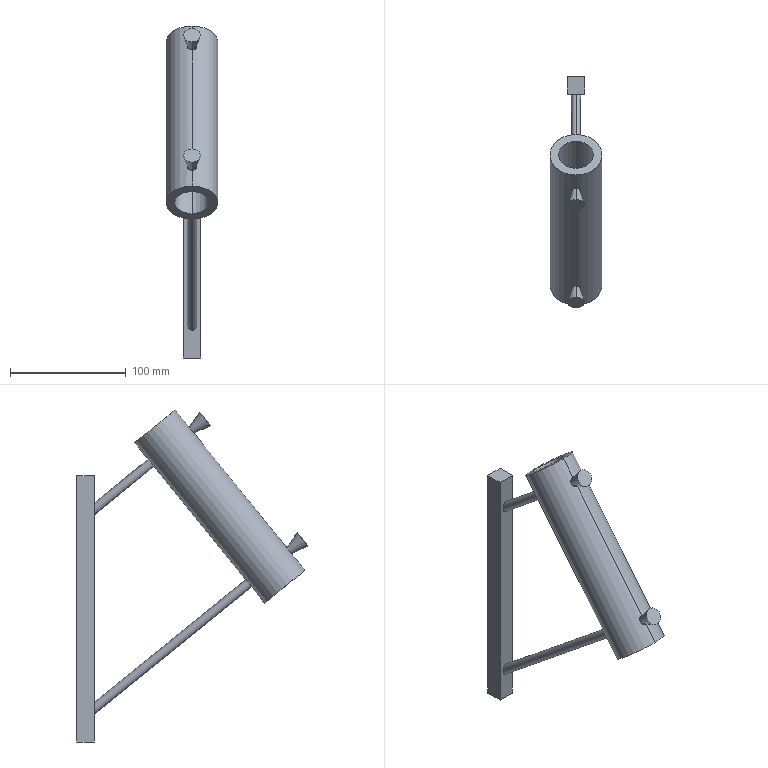Part | SolidWorks | features ICE 7, Cut 1, Extrusion 1 | 1 solid | 34 faces | box 45 x 200.096 x 286.61 mm | volume 222734 mm3 | cylinder 16 | plane 14 | cone 4 | commonest cylinder face diameters 8 x5 8.4 x4 8.2 x2 30 x2 45 x2 8.948 x1
STEP:
#1=CARTESIAN_POINT('',(-7.5,-176.098,143.559));
#2=VERTEX_POINT('',#1);
#3=CARTESIAN_POINT('',(-7.5,-152.784,124.679));
#4=VERTEX_POINT('',#3);
#5=CARTESIAN_POINT('',(-7.5,-164.441,134.119));
#6=DIRECTION('',(0.,-0.6293,-0.7771));
#7=DIRECTION('',(0.,0.7771,-0.6293));
#8=AXIS2_PLACEMENT_3D('',#5,#6,#7);
#9=CIRCLE('',#8,15.);
#10=EDGE_CURVE('',#2,#4,#9,.T.);
#11=ORIENTED_EDGE('',*,*,#10,.T.);
#12=CARTESIAN_POINT('',(-7.5,-40.765,263.011));
#13=VERTEX_POINT('',#12);
#14=CARTESIAN_POINT('',(-7.5,-162.224,113.022));
#15=DIRECTION('',(0.,0.6293,0.7771));
#16=VECTOR('',#15,1000.);
#17=LINE('',#14,#16);
#18=EDGE_CURVE('',#4,#13,#17,.T.);
#19=ORIENTED_EDGE('',*,*,#18,.T.);
#20=CARTESIAN_POINT('',(-7.5,-64.079,281.891));
#21=VERTEX_POINT('',#20);
#22=CARTESIAN_POINT('',(-7.5,-52.422,272.451));
#23=DIRECTION('',(0.,0.6293,0.7771));
#24=DIRECTION('',(0.,-0.7771,0.6293));
#25=AXIS2_PLACEMENT_3D('',#22,#23,#24);
#26=CIRCLE('',#25,15.);
#27=EDGE_CURVE('',#13,#21,#26,.T.);
#28=ORIENTED_EDGE('',*,*,#27,.T.);
#29=CARTESIAN_POINT('',(-7.5,-185.538,131.901));
#30=DIRECTION('',(0.,0.6293,0.7771));
#31=VECTOR('',#30,1000.);
#32=LINE('',#29,#31);
#33=EDGE_CURVE('',#2,#21,#32,.T.);
#34=ORIENTED_EDGE('',*,*,#33,.F.);
#35=EDGE_LOOP('',(#11,#19,#28,#34));
#36=FACE_OUTER_BOUND('',#35,.T.);
#37=CARTESIAN_POINT('',(-7.5,-173.881,122.462));
#38=DIRECTION('',(0.,0.6293,0.7771));
#39=DIRECTION('',(0.,-0.7771,0.6293));
#40=AXIS2_PLACEMENT_3D('',#37,#38,#39);
#41=CYLINDRICAL_SURFACE('',#40,15.);
#42=ADVANCED_FACE('',(#36),#41,.F.);
#43=CARTESIAN_POINT('',(-7.5,-165.539,160.642));
#44=VERTEX_POINT('',#43);
#45=CARTESIAN_POINT('',(-7.5,-163.022,163.751));
#46=VERTEX_POINT('',#45);
#47=CARTESIAN_POINT('',(-7.5,-164.281,162.197));
#48=DIRECTION('',(0.,-0.7771,0.6293));
#49=DIRECTION('',(0.,-0.6293,-0.7771));
#50=AXIS2_PLACEMENT_3D('',#47,#48,#49);
#51=CIRCLE('',#50,2.);
#52=EDGE_CURVE('',#44,#46,#51,.T.);
#53=ORIENTED_EDGE('',*,*,#52,.T.);
#54=CARTESIAN_POINT('',(-7.5,-175.192,180.502));
#55=VERTEX_POINT('',#54);
#56=CARTESIAN_POINT('',(-7.5,-163.022,163.751));
#57=DIRECTION('',(0.,-0.5878,0.809));
#58=VECTOR('',#57,1000.);
#59=LINE('',#56,#58);
#60=EDGE_CURVE('',#46,#55,#59,.T.);
#61=ORIENTED_EDGE('',*,*,#60,.T.);
#62=CARTESIAN_POINT('',(-7.5,-184.455,169.064));
#63=VERTEX_POINT('',#62);
#64=CARTESIAN_POINT('',(-7.5,-179.823,174.783));
#65=DIRECTION('',(0.,-0.7771,0.6293));
#66=DIRECTION('',(0.,-0.6293,-0.7771));
#67=AXIS2_PLACEMENT_3D('',#64,#65,#66);
#68=CIRCLE('',#67,7.359);
#69=EDGE_CURVE('',#63,#55,#68,.T.);
#70=ORIENTED_EDGE('',*,*,#69,.F.);
#71=CARTESIAN_POINT('',(-7.5,-165.539,160.642));
#72=DIRECTION('',(0.,-0.9135,0.4067));
#73=VECTOR('',#72,1000.);
#74=LINE('',#71,#73);
#75=EDGE_CURVE('',#44,#63,#74,.T.);
#76=ORIENTED_EDGE('',*,*,#75,.F.);
#77=EDGE_LOOP('',(#53,#61,#70,#76));
#78=FACE_OUTER_BOUND('',#77,.T.);
#79=CARTESIAN_POINT('',(-7.5,-164.281,162.197));
#80=DIRECTION('',(0.,-0.7771,0.6293));
#81=DIRECTION('',(0.,-0.6293,-0.7771));
#82=AXIS2_PLACEMENT_3D('',#79,#80,#81);
#83=CONICAL_SURFACE('',#82,2.,0.2618);
#84=ADVANCED_FACE('',(#78),#83,.T.);
#85=CARTESIAN_POINT('',(-7.5,-81.392,264.555));
#86=VERTEX_POINT('',#85);
#87=CARTESIAN_POINT('',(-7.5,-78.875,267.664));
#88=VERTEX_POINT('',#87);
#89=CARTESIAN_POINT('',(-7.5,-80.134,266.109));
#90=DIRECTION('',(0.,-0.7771,0.6293));
#91=DIRECTION('',(0.,-0.6293,-0.7771));
#92=AXIS2_PLACEMENT_3D('',#89,#90,#91);
#93=CIRCLE('',#92,2.);
#94=EDGE_CURVE('',#86,#88,#93,.T.);
#95=ORIENTED_EDGE('',*,*,#94,.T.);
#96=CARTESIAN_POINT('',(-7.5,-91.046,284.415));
#97=VERTEX_POINT('',#96);
#98=CARTESIAN_POINT('',(-7.5,-78.875,267.664));
#99=DIRECTION('',(0.,-0.5878,0.809));
#100=VECTOR('',#99,1000.);
#101=LINE('',#98,#100);
#102=EDGE_CURVE('',#88,#97,#101,.T.);
#103=ORIENTED_EDGE('',*,*,#102,.T.);
#104=CARTESIAN_POINT('',(-7.5,-100.308,272.977));
#105=VERTEX_POINT('',#104);
#106=CARTESIAN_POINT('',(-7.5,-95.677,278.696));
#107=DIRECTION('',(0.,-0.7771,0.6293));
#108=DIRECTION('',(0.,-0.6293,-0.7771));
#109=AXIS2_PLACEMENT_3D('',#106,#107,#108);
#110=CIRCLE('',#109,7.359);
#111=EDGE_CURVE('',#105,#97,#110,.T.);
#112=ORIENTED_EDGE('',*,*,#111,.F.);
#113=CARTESIAN_POINT('',(-7.5,-81.392,264.555));
#114=DIRECTION('',(0.,-0.9135,0.4067));
#115=VECTOR('',#114,1000.);
#116=LINE('',#113,#115);
#117=EDGE_CURVE('',#86,#105,#116,.T.);
#118=ORIENTED_EDGE('',*,*,#117,.F.);
#119=EDGE_LOOP('',(#95,#103,#112,#118));
#120=FACE_OUTER_BOUND('',#119,.T.);
#121=CARTESIAN_POINT('',(-7.5,-80.134,266.109));
#122=DIRECTION('',(0.,-0.7771,0.6293));
#123=DIRECTION('',(0.,-0.6293,-0.7771));
#124=AXIS2_PLACEMENT_3D('',#121,#122,#123);
#125=CONICAL_SURFACE('',#124,2.,0.2618);
#126=ADVANCED_FACE('',(#120),#125,.T.);
#127=CARTESIAN_POINT('',(-7.5,-77.491,269.373));
#128=VERTEX_POINT('',#127);
#129=CARTESIAN_POINT('',(-7.5,-82.777,262.845));
#130=VERTEX_POINT('',#129);
#131=CARTESIAN_POINT('',(-7.5,-80.134,266.109));
#132=DIRECTION('',(0.,-0.7771,0.6293));
#133=DIRECTION('',(0.,-0.6293,-0.7771));
#134=AXIS2_PLACEMENT_3D('',#131,#132,#133);
#135=CIRCLE('',#134,4.2);
#136=EDGE_CURVE('',#128,#130,#135,.T.);
#137=ORIENTED_EDGE('',*,*,#136,.F.);
#138=CARTESIAN_POINT('',(-7.5,-81.341,272.491));
#139=VERTEX_POINT('',#138);
#140=CARTESIAN_POINT('',(-7.5,-77.491,269.373));
#141=DIRECTION('',(0.,-0.7771,0.6293));
#142=VECTOR('',#141,1000.);
#143=LINE('',#140,#142);
#144=EDGE_CURVE('',#128,#139,#143,.T.);
#145=ORIENTED_EDGE('',*,*,#144,.T.);
#146=CARTESIAN_POINT('',(-7.5,-86.628,265.963));
#147=VERTEX_POINT('',#146);
#148=CARTESIAN_POINT('',(-7.5,-86.628,265.963));
#149=CARTESIAN_POINT('',(-7.778,-86.628,265.963));
#150=CARTESIAN_POINT('',(-8.052,-86.606,265.981));
#151=CARTESIAN_POINT('',(-8.589,-86.524,266.052));
#152=CARTESIAN_POINT('',(-8.856,-86.461,266.106));
#153=CARTESIAN_POINT('',(-9.365,-86.3,266.247));
#154=CARTESIAN_POINT('',(-9.606,-86.202,266.334));
#155=CARTESIAN_POINT('',(-10.062,-85.973,266.541));
#156=CARTESIAN_POINT('',(-10.277,-85.842,266.662));
#157=CARTESIAN_POINT('',(-10.664,-85.558,266.93));
#158=CARTESIAN_POINT('',(-10.837,-85.406,267.078));
#159=CARTESIAN_POINT('',(-11.144,-85.079,267.404));
#160=CARTESIAN_POINT('',(-11.275,-84.909,267.58));
#161=CARTESIAN_POINT('',(-11.484,-84.562,267.949));
#162=CARTESIAN_POINT('',(-11.565,-84.384,268.146));
#163=CARTESIAN_POINT('',(-11.673,-84.027,268.555));
#164=CARTESIAN_POINT('',(-11.7,-83.851,268.764));
#165=CARTESIAN_POINT('',(-11.7,-83.505,269.191));
#166=CARTESIAN_POINT('',(-11.673,-83.334,269.411));
#167=CARTESIAN_POINT('',(-11.565,-83.01,269.842));
#168=CARTESIAN_POINT('',(-11.486,-82.857,270.055));
#169=CARTESIAN_POINT('',(-11.275,-82.565,270.474));
#170=CARTESIAN_POINT('',(-11.143,-82.428,270.679));
#171=CARTESIAN_POINT('',(-10.839,-82.179,271.062));
#172=CARTESIAN_POINT('',(-10.665,-82.065,271.244));
#173=CARTESIAN_POINT('',(-10.274,-81.86,271.58));
#174=CARTESIAN_POINT('',(-10.063,-81.771,271.731));
#175=CARTESIAN_POINT('',(-9.609,-81.616,271.997));
#176=CARTESIAN_POINT('',(-9.363,-81.55,272.113));
#177=CARTESIAN_POINT('',(-8.855,-81.446,272.3));
#178=CARTESIAN_POINT('',(-8.593,-81.407,272.371));
#179=CARTESIAN_POINT('',(-8.053,-81.355,272.467));
#180=CARTESIAN_POINT('',(-7.774,-81.341,272.491));
#181=CARTESIAN_POINT('',(-7.5,-81.341,272.491));
#182=B_SPLINE_CURVE_WITH_KNOTS('',3,(#148,#149,#150,#151,#152,#153,#154,#155,#156,#157,#158,#159,#160,#161,#162,#163,#164,#165,#166,#167,#168,#169,#170,#171,#172,#173,#174,#175,#176,#177,#178,#179,#180,#181),.UNSPECIFIED.,.F.,.F.,(4,2,2,2,2,2,2,2,2,2,2,2,2,2,2,2,4),(0.,0.0008225,0.001645,0.002468,0.00329,0.004113,0.004935,0.005758,0.00658,0.007403,0.008225,0.009048,0.00987,0.01069,0.01152,0.01234,0.01316),.UNSPECIFIED.);
#183=EDGE_CURVE('',#147,#139,#182,.T.);
#184=ORIENTED_EDGE('',*,*,#183,.F.);
#185=CARTESIAN_POINT('',(-7.5,-82.777,262.845));
#186=DIRECTION('',(0.,-0.7771,0.6293));
#187=VECTOR('',#186,1000.);
#188=LINE('',#185,#187);
#189=EDGE_CURVE('',#130,#147,#188,.T.);
#190=ORIENTED_EDGE('',*,*,#189,.F.);
#191=EDGE_LOOP('',(#137,#145,#184,#190));
#192=FACE_OUTER_BOUND('',#191,.T.);
#193=CARTESIAN_POINT('',(-7.5,-80.134,266.109));
#194=DIRECTION('',(0.,-0.7771,0.6293));
#195=DIRECTION('',(0.,-0.6293,-0.7771));
#196=AXIS2_PLACEMENT_3D('',#193,#194,#195);
#197=CYLINDRICAL_SURFACE('',#196,4.2);
#198=ADVANCED_FACE('',(#192),#197,.F.);
#199=CARTESIAN_POINT('',(-7.5,-161.637,165.461));
#200=VERTEX_POINT('',#199);
#201=CARTESIAN_POINT('',(-7.5,-166.924,158.933));
#202=VERTEX_POINT('',#201);
#203=CARTESIAN_POINT('',(-7.5,-164.281,162.197));
#204=DIRECTION('',(0.,-0.7771,0.6293));
#205=DIRECTION('',(0.,-0.6293,-0.7771));
#206=AXIS2_PLACEMENT_3D('',#203,#204,#205);
#207=CIRCLE('',#206,4.2);
#208=EDGE_CURVE('',#200,#202,#207,.T.);
#209=ORIENTED_EDGE('',*,*,#208,.F.);
#210=CARTESIAN_POINT('',(-7.5,-165.488,168.579));
#211=VERTEX_POINT('',#210);
#212=CARTESIAN_POINT('',(-7.5,-161.637,165.461));
#213=DIRECTION('',(0.,-0.7771,0.6293));
#214=VECTOR('',#213,1000.);
#215=LINE('',#212,#214);
#216=EDGE_CURVE('',#200,#211,#215,.T.);
#217=ORIENTED_EDGE('',*,*,#216,.T.);
#218=CARTESIAN_POINT('',(-7.5,-170.774,162.051));
#219=VERTEX_POINT('',#218);
#220=CARTESIAN_POINT('',(-7.5,-170.774,162.051));
#221=CARTESIAN_POINT('',(-7.778,-170.774,162.051));
#222=CARTESIAN_POINT('',(-8.052,-170.753,162.069));
#223=CARTESIAN_POINT('',(-8.589,-170.67,162.14));
#224=CARTESIAN_POINT('',(-8.856,-170.608,162.194));
#225=CARTESIAN_POINT('',(-9.365,-170.447,162.335));
#226=CARTESIAN_POINT('',(-9.606,-170.349,162.421));
#227=CARTESIAN_POINT('',(-10.062,-170.12,162.628));
#228=CARTESIAN_POINT('',(-10.277,-169.988,162.749));
#229=CARTESIAN_POINT('',(-10.664,-169.705,163.018));
#230=CARTESIAN_POINT('',(-10.837,-169.552,163.165));
#231=CARTESIAN_POINT('',(-11.144,-169.226,163.492));
#232=CARTESIAN_POINT('',(-11.275,-169.056,163.667));
#233=CARTESIAN_POINT('',(-11.484,-168.709,164.037));
#234=CARTESIAN_POINT('',(-11.565,-168.531,164.234));
#235=CARTESIAN_POINT('',(-11.673,-168.173,164.643));
#236=CARTESIAN_POINT('',(-11.7,-167.998,164.851));
#237=CARTESIAN_POINT('',(-11.7,-167.652,165.278));
#238=CARTESIAN_POINT('',(-11.673,-167.481,165.498));
#239=CARTESIAN_POINT('',(-11.565,-167.157,165.93));
#240=CARTESIAN_POINT('',(-11.486,-167.003,166.143));
#241=CARTESIAN_POINT('',(-11.275,-166.711,166.562));
#242=CARTESIAN_POINT('',(-11.143,-166.575,166.766));
#243=CARTESIAN_POINT('',(-10.839,-166.326,167.149));
#244=CARTESIAN_POINT('',(-10.665,-166.212,167.331));
#245=CARTESIAN_POINT('',(-10.274,-166.006,167.667));
#246=CARTESIAN_POINT('',(-10.063,-165.917,167.818));
#247=CARTESIAN_POINT('',(-9.609,-165.763,168.084));
#248=CARTESIAN_POINT('',(-9.363,-165.697,168.201));
#249=CARTESIAN_POINT('',(-8.855,-165.593,168.387));
#250=CARTESIAN_POINT('',(-8.593,-165.554,168.458));
#251=CARTESIAN_POINT('',(-8.053,-165.501,168.554));
#252=CARTESIAN_POINT('',(-7.774,-165.488,168.579));
#253=CARTESIAN_POINT('',(-7.5,-165.488,168.579));
#254=B_SPLINE_CURVE_WITH_KNOTS('',3,(#220,#221,#222,#223,#224,#225,#226,#227,#228,#229,#230,#231,#232,#233,#234,#235,#236,#237,#238,#239,#240,#241,#242,#243,#244,#245,#246,#247,#248,#249,#250,#251,#252,#253),.UNSPECIFIED.,.F.,.F.,(4,2,2,2,2,2,2,2,2,2,2,2,2,2,2,2,4),(0.,0.0008225,0.001645,0.002468,0.00329,0.004113,0.004935,0.005758,0.00658,0.007403,0.008225,0.009048,0.00987,0.01069,0.01152,0.01234,0.01316),.UNSPECIFIED.);
#255=EDGE_CURVE('',#219,#211,#254,.T.);
#256=ORIENTED_EDGE('',*,*,#255,.F.);
#257=CARTESIAN_POINT('',(-7.5,-166.924,158.933));
#258=DIRECTION('',(0.,-0.7771,0.6293));
#259=VECTOR('',#258,1000.);
#260=LINE('',#257,#259);
#261=EDGE_CURVE('',#202,#219,#260,.T.);
#262=ORIENTED_EDGE('',*,*,#261,.F.);
#263=EDGE_LOOP('',(#209,#217,#256,#262));
#264=FACE_OUTER_BOUND('',#263,.T.);
#265=CARTESIAN_POINT('',(-7.5,-164.281,162.197));
#266=DIRECTION('',(0.,-0.7771,0.6293));
#267=DIRECTION('',(0.,-0.6293,-0.7771));
#268=AXIS2_PLACEMENT_3D('',#265,#266,#267);
#269=CYLINDRICAL_SURFACE('',#268,4.2);
#270=ADVANCED_FACE('',(#264),#269,.F.);
#271=CARTESIAN_POINT('',(-7.5,-146.956,119.959));
#272=VERTEX_POINT('',#271);
#273=CARTESIAN_POINT('',(-7.5,-181.927,148.278));
#274=VERTEX_POINT('',#273);
#275=CARTESIAN_POINT('',(-7.5,-164.441,134.119));
#276=DIRECTION('',(0.,-0.6293,-0.7771));
#277=DIRECTION('',(0.,0.7771,-0.6293));
#278=AXIS2_PLACEMENT_3D('',#275,#276,#277);
#279=CIRCLE('',#278,22.5);
#280=EDGE_CURVE('',#272,#274,#279,.T.);
#281=ORIENTED_EDGE('',*,*,#280,.F.);
#282=CARTESIAN_POINT('',(-7.5,-135.677,133.887));
#283=VERTEX_POINT('',#282);
#284=CARTESIAN_POINT('',(-7.5,-146.956,119.959));
#285=DIRECTION('',(0.,0.6293,0.7771));
#286=VECTOR('',#285,1000.);
#287=LINE('',#284,#286);
#288=EDGE_CURVE('',#272,#283,#287,.T.);
#289=ORIENTED_EDGE('',*,*,#288,.T.);
#290=CARTESIAN_POINT('',(-7.5,-130.642,140.104));
#291=VERTEX_POINT('',#290);
#292=CARTESIAN_POINT('',(-7.5,-135.677,133.887));
#293=CARTESIAN_POINT('',(-7.235,-135.677,133.887));
#294=CARTESIAN_POINT('',(-6.975,-135.664,133.91));
#295=CARTESIAN_POINT('',(-6.463,-135.614,134.001));
#296=CARTESIAN_POINT('',(-6.208,-135.576,134.069));
#297=CARTESIAN_POINT('',(-5.724,-135.475,134.246));
#298=CARTESIAN_POINT('',(-5.495,-135.413,134.354));
#299=CARTESIAN_POINT('',(-5.06,-135.263,134.607));
#300=CARTESIAN_POINT('',(-4.855,-135.176,134.753));
#301=CARTESIAN_POINT('',(-4.487,-134.98,135.068));
#302=CARTESIAN_POINT('',(-4.321,-134.872,135.239));
#303=CARTESIAN_POINT('',(-4.029,-134.631,135.606));
#304=CARTESIAN_POINT('',(-3.905,-134.5,135.799));
#305=CARTESIAN_POINT('',(-3.706,-134.223,136.194));
#306=CARTESIAN_POINT('',(-3.628,-134.075,136.399));
#307=CARTESIAN_POINT('',(-3.526,-133.764,136.812));
#308=CARTESIAN_POINT('',(-3.5,-133.604,137.017));
#309=CARTESIAN_POINT('',(-3.5,-133.275,137.423));
#310=CARTESIAN_POINT('',(-3.526,-133.104,137.627));
#311=CARTESIAN_POINT('',(-3.628,-132.766,138.014));
#312=CARTESIAN_POINT('',(-3.704,-132.599,138.2));
#313=CARTESIAN_POINT('',(-3.905,-132.268,138.556));
#314=CARTESIAN_POINT('',(-4.03,-132.105,138.724));
#315=CARTESIAN_POINT('',(-4.32,-131.799,139.033));
#316=CARTESIAN_POINT('',(-4.486,-131.654,139.176));
#317=CARTESIAN_POINT('',(-4.858,-131.383,139.436));
#318=CARTESIAN_POINT('',(-5.059,-131.261,139.549));
#319=CARTESIAN_POINT('',(-5.492,-131.045,139.747));
#320=CARTESIAN_POINT('',(-5.726,-130.951,139.832));
#321=CARTESIAN_POINT('',(-6.21,-130.799,139.968));
#322=CARTESIAN_POINT('',(-6.459,-130.741,140.018));
#323=CARTESIAN_POINT('',(-6.973,-130.662,140.087));
#324=CARTESIAN_POINT('',(-7.239,-130.642,140.104));
#325=CARTESIAN_POINT('',(-7.5,-130.642,140.104));
#326=B_SPLINE_CURVE_WITH_KNOTS('',3,(#292,#293,#294,#295,#296,#297,#298,#299,#300,#301,#302,#303,#304,#305,#306,#307,#308,#309,#310,#311,#312,#313,#314,#315,#316,#317,#318,#319,#320,#321,#322,#323,#324,#325),.UNSPECIFIED.,.F.,.F.,(4,2,2,2,2,2,2,2,2,2,2,2,2,2,2,2,4),(0.,0.0007832,0.001566,0.00235,0.003133,0.003916,0.004699,0.005482,0.006265,0.007049,0.007832,0.008615,0.009398,0.01018,0.01096,0.01175,0.01253),.UNSPECIFIED.);
#327=EDGE_CURVE('',#283,#291,#326,.T.);
#328=ORIENTED_EDGE('',*,*,#327,.T.);
#329=CARTESIAN_POINT('',(-7.5,-51.53,237.799));
#330=VERTEX_POINT('',#329);
#331=CARTESIAN_POINT('',(-7.5,-146.956,119.959));
#332=DIRECTION('',(0.,0.6293,0.7771));
#333=VECTOR('',#332,1000.);
#334=LINE('',#331,#333);
#335=EDGE_CURVE('',#291,#330,#334,.T.);
#336=ORIENTED_EDGE('',*,*,#335,.T.);
#337=CARTESIAN_POINT('',(-7.5,-46.496,244.017));
#338=VERTEX_POINT('',#337);
#339=CARTESIAN_POINT('',(-7.5,-51.53,237.799));
#340=CARTESIAN_POINT('',(-7.235,-51.53,237.799));
#341=CARTESIAN_POINT('',(-6.975,-51.517,237.823));
#342=CARTESIAN_POINT('',(-6.463,-51.467,237.913));
#343=CARTESIAN_POINT('',(-6.208,-51.429,237.981));
#344=CARTESIAN_POINT('',(-5.724,-51.328,238.158));
#345=CARTESIAN_POINT('',(-5.495,-51.266,238.266));
#346=CARTESIAN_POINT('',(-5.06,-51.117,238.519));
#347=CARTESIAN_POINT('',(-4.855,-51.029,238.665));
#348=CARTESIAN_POINT('',(-4.487,-50.834,238.981));
#349=CARTESIAN_POINT('',(-4.321,-50.725,239.152));
#350=CARTESIAN_POINT('',(-4.029,-50.484,239.519));
#351=CARTESIAN_POINT('',(-3.905,-50.353,239.712));
#352=CARTESIAN_POINT('',(-3.706,-50.076,240.106));
#353=CARTESIAN_POINT('',(-3.628,-49.928,240.311));
#354=CARTESIAN_POINT('',(-3.526,-49.617,240.724));
#355=CARTESIAN_POINT('',(-3.5,-49.457,240.929));
#356=CARTESIAN_POINT('',(-3.5,-49.128,241.336));
#357=CARTESIAN_POINT('',(-3.526,-48.957,241.539));
#358=CARTESIAN_POINT('',(-3.628,-48.62,241.927));
#359=CARTESIAN_POINT('',(-3.704,-48.452,242.112));
#360=CARTESIAN_POINT('',(-3.905,-48.121,242.468));
#361=CARTESIAN_POINT('',(-4.03,-47.959,242.637));
#362=CARTESIAN_POINT('',(-4.32,-47.653,242.946));
#363=CARTESIAN_POINT('',(-4.486,-47.507,243.089));
#364=CARTESIAN_POINT('',(-4.858,-47.236,243.348));
#365=CARTESIAN_POINT('',(-5.059,-47.114,243.462));
#366=CARTESIAN_POINT('',(-5.492,-46.899,243.66));
#367=CARTESIAN_POINT('',(-5.726,-46.804,243.745));
#368=CARTESIAN_POINT('',(-6.21,-46.652,243.88));
#369=CARTESIAN_POINT('',(-6.459,-46.594,243.931));
#370=CARTESIAN_POINT('',(-6.973,-46.516,243.999));
#371=CARTESIAN_POINT('',(-7.239,-46.496,244.017));
#372=CARTESIAN_POINT('',(-7.5,-46.496,244.017));
#373=B_SPLINE_CURVE_WITH_KNOTS('',3,(#339,#340,#341,#342,#343,#344,#345,#346,#347,#348,#349,#350,#351,#352,#353,#354,#355,#356,#357,#358,#359,#360,#361,#362,#363,#364,#365,#366,#367,#368,#369,#370,#371,#372),.UNSPECIFIED.,.F.,.F.,(4,2,2,2,2,2,2,2,2,2,2,2,2,2,2,2,4),(0.,0.0007832,0.001566,0.00235,0.003133,0.003916,0.004699,0.005482,0.006265,0.007049,0.007832,0.008615,0.009398,0.01018,0.01096,0.01175,0.01253),.UNSPECIFIED.);
#374=EDGE_CURVE('',#330,#338,#373,.T.);
#375=ORIENTED_EDGE('',*,*,#374,.T.);
#376=CARTESIAN_POINT('',(-7.5,-34.936,258.291));
#377=VERTEX_POINT('',#376);
#378=CARTESIAN_POINT('',(-7.5,-146.956,119.959));
#379=DIRECTION('',(0.,0.6293,0.7771));
#380=VECTOR('',#379,1000.);
#381=LINE('',#378,#380);
#382=EDGE_CURVE('',#338,#377,#381,.T.);
#383=ORIENTED_EDGE('',*,*,#382,.T.);
#384=CARTESIAN_POINT('',(-7.5,-69.908,286.61));
#385=VERTEX_POINT('',#384);
#386=CARTESIAN_POINT('',(-7.5,-52.422,272.451));
#387=DIRECTION('',(0.,-0.6293,-0.7771));
#388=DIRECTION('',(0.,0.7771,-0.6293));
#389=AXIS2_PLACEMENT_3D('',#386,#387,#388);
#390=CIRCLE('',#389,22.5);
#391=EDGE_CURVE('',#377,#385,#390,.T.);
#392=ORIENTED_EDGE('',*,*,#391,.T.);
#393=CARTESIAN_POINT('',(-7.5,-181.927,148.278));
#394=DIRECTION('',(0.,0.6293,0.7771));
#395=VECTOR('',#394,1000.);
#396=LINE('',#393,#395);
#397=EDGE_CURVE('',#139,#385,#396,.T.);
#398=ORIENTED_EDGE('',*,*,#397,.F.);
#399=CARTESIAN_POINT('',(-7.5,-81.341,272.491));
#400=CARTESIAN_POINT('',(-7.226,-81.341,272.491));
#401=CARTESIAN_POINT('',(-6.953,-81.354,272.468));
#402=CARTESIAN_POINT('',(-6.409,-81.407,272.371));
#403=CARTESIAN_POINT('',(-6.145,-81.446,272.299));
#404=CARTESIAN_POINT('',(-5.639,-81.55,272.114));
#405=CARTESIAN_POINT('',(-5.394,-81.615,271.998));
#406=CARTESIAN_POINT('',(-4.937,-81.771,271.73));
#407=CARTESIAN_POINT('',(-4.726,-81.86,271.58));
#408=CARTESIAN_POINT('',(-4.338,-82.063,271.247));
#409=CARTESIAN_POINT('',(-4.161,-82.179,271.063));
#410=CARTESIAN_POINT('',(-3.857,-82.428,270.679));
#411=CARTESIAN_POINT('',(-3.728,-82.562,270.478));
#412=CARTESIAN_POINT('',(-3.516,-82.854,270.059));
#413=CARTESIAN_POINT('',(-3.435,-83.01,269.843));
#414=CARTESIAN_POINT('',(-3.328,-83.332,269.413));
#415=CARTESIAN_POINT('',(-3.3,-83.501,269.196));
#416=CARTESIAN_POINT('',(-3.3,-83.85,268.765));
#417=CARTESIAN_POINT('',(-3.327,-84.026,268.556));
#418=CARTESIAN_POINT('',(-3.434,-84.38,268.15));
#419=CARTESIAN_POINT('',(-3.515,-84.56,267.952));
#420=CARTESIAN_POINT('',(-3.725,-84.908,267.58));
#421=CARTESIAN_POINT('',(-3.854,-85.077,267.407));
#422=CARTESIAN_POINT('',(-4.159,-85.402,267.082));
#423=CARTESIAN_POINT('',(-4.335,-85.557,266.931));
#424=CARTESIAN_POINT('',(-4.721,-85.841,266.663));
#425=CARTESIAN_POINT('',(-4.932,-85.97,266.544));
#426=CARTESIAN_POINT('',(-5.392,-86.201,266.335));
#427=CARTESIAN_POINT('',(-5.634,-86.3,266.248));
#428=CARTESIAN_POINT('',(-6.139,-86.46,266.107));
#429=CARTESIAN_POINT('',(-6.405,-86.523,266.053));
#430=CARTESIAN_POINT('',(-6.947,-86.606,265.981));
#431=CARTESIAN_POINT('',(-7.222,-86.628,265.963));
#432=CARTESIAN_POINT('',(-7.5,-86.628,265.963));
#433=B_SPLINE_CURVE_WITH_KNOTS('',3,(#399,#400,#401,#402,#403,#404,#405,#406,#407,#408,#409,#410,#411,#412,#413,#414,#415,#416,#417,#418,#419,#420,#421,#422,#423,#424,#425,#426,#427,#428,#429,#430,#431,#432),.UNSPECIFIED.,.F.,.F.,(4,2,2,2,2,2,2,2,2,2,2,2,2,2,2,2,4),(0.01316,0.01398,0.0148,0.01563,0.01645,0.01727,0.01809,0.01892,0.01974,0.02056,0.02138,0.02221,0.02303,0.02385,0.02467,0.02549,0.02632),.UNSPECIFIED.);
#434=EDGE_CURVE('',#139,#147,#433,.T.);
#435=ORIENTED_EDGE('',*,*,#434,.T.);
#436=CARTESIAN_POINT('',(-7.5,-181.927,148.278));
#437=DIRECTION('',(0.,0.6293,0.7771));
#438=VECTOR('',#437,1000.);
#439=LINE('',#436,#438);
#440=EDGE_CURVE('',#211,#147,#439,.T.);
#441=ORIENTED_EDGE('',*,*,#440,.F.);
#442=CARTESIAN_POINT('',(-7.5,-165.488,168.579));
#443=CARTESIAN_POINT('',(-7.226,-165.488,168.579));
#444=CARTESIAN_POINT('',(-6.953,-165.501,168.555));
#445=CARTESIAN_POINT('',(-6.409,-165.554,168.459));
#446=CARTESIAN_POINT('',(-6.145,-165.593,168.387));
#447=CARTESIAN_POINT('',(-5.639,-165.697,168.201));
#448=CARTESIAN_POINT('',(-5.394,-165.762,168.086));
#449=CARTESIAN_POINT('',(-4.937,-165.917,167.818));
#450=CARTESIAN_POINT('',(-4.726,-166.007,167.667));
#451=CARTESIAN_POINT('',(-4.338,-166.21,167.334));
#452=CARTESIAN_POINT('',(-4.161,-166.325,167.15));
#453=CARTESIAN_POINT('',(-3.857,-166.574,166.766));
#454=CARTESIAN_POINT('',(-3.728,-166.709,166.566));
#455=CARTESIAN_POINT('',(-3.516,-167.001,166.146));
#456=CARTESIAN_POINT('',(-3.435,-167.157,165.93));
#457=CARTESIAN_POINT('',(-3.328,-167.479,165.5));
#458=CARTESIAN_POINT('',(-3.3,-167.648,165.283));
#459=CARTESIAN_POINT('',(-3.3,-167.997,164.852));
#460=CARTESIAN_POINT('',(-3.327,-168.173,164.643));
#461=CARTESIAN_POINT('',(-3.434,-168.527,164.238));
#462=CARTESIAN_POINT('',(-3.515,-168.707,164.039));
#463=CARTESIAN_POINT('',(-3.725,-169.055,163.668));
#464=CARTESIAN_POINT('',(-3.854,-169.224,163.494));
#465=CARTESIAN_POINT('',(-4.159,-169.549,163.169));
#466=CARTESIAN_POINT('',(-4.335,-169.704,163.018));
#467=CARTESIAN_POINT('',(-4.721,-169.987,162.75));
#468=CARTESIAN_POINT('',(-4.932,-170.117,162.631));
#469=CARTESIAN_POINT('',(-5.392,-170.348,162.422));
#470=CARTESIAN_POINT('',(-5.634,-170.446,162.335));
#471=CARTESIAN_POINT('',(-6.139,-170.607,162.195));
#472=CARTESIAN_POINT('',(-6.405,-170.669,162.141));
#473=CARTESIAN_POINT('',(-6.947,-170.753,162.069));
#474=CARTESIAN_POINT('',(-7.222,-170.774,162.051));
#475=CARTESIAN_POINT('',(-7.5,-170.774,162.051));
#476=B_SPLINE_CURVE_WITH_KNOTS('',3,(#442,#443,#444,#445,#446,#447,#448,#449,#450,#451,#452,#453,#454,#455,#456,#457,#458,#459,#460,#461,#462,#463,#464,#465,#466,#467,#468,#469,#470,#471,#472,#473,#474,#475),.UNSPECIFIED.,.F.,.F.,(4,2,2,2,2,2,2,2,2,2,2,2,2,2,2,2,4),(0.01316,0.01398,0.0148,0.01563,0.01645,0.01727,0.01809,0.01892,0.01974,0.02056,0.02138,0.02221,0.02303,0.02385,0.02467,0.02549,0.02632),.UNSPECIFIED.);
#477=EDGE_CURVE('',#211,#219,#476,.T.);
#478=ORIENTED_EDGE('',*,*,#477,.T.);
#479=CARTESIAN_POINT('',(-7.5,-181.927,148.278));
#480=DIRECTION('',(0.,0.6293,0.7771));
#481=VECTOR('',#480,1000.);
#482=LINE('',#479,#481);
#483=EDGE_CURVE('',#274,#219,#482,.T.);
#484=ORIENTED_EDGE('',*,*,#483,.F.);
#485=EDGE_LOOP('',(#281,#289,#328,#336,#375,#383,#392,#398,#435,#441,#478,#484));
#486=FACE_OUTER_BOUND('',#485,.T.);
#487=CARTESIAN_POINT('',(-7.5,-164.441,134.119));
#488=DIRECTION('',(0.,0.6293,0.7771));
#489=DIRECTION('',(0.,-0.7771,0.6293));
#490=AXIS2_PLACEMENT_3D('',#487,#488,#489);
#491=CYLINDRICAL_SURFACE('',#490,22.5);
#492=ADVANCED_FACE('',(#486),#491,.T.);
#493=CARTESIAN_POINT('',(-7.5,6.443,18.672));
#494=VERTEX_POINT('',#493);
#495=CARTESIAN_POINT('',(-7.5,11.603,25.045));
#496=VERTEX_POINT('',#495);
#497=CARTESIAN_POINT('',(-7.5,9.023,21.858));
#498=DIRECTION('',(0.,0.7771,-0.6293));
#499=DIRECTION('',(0.,0.6293,0.7771));
#500=AXIS2_PLACEMENT_3D('',#497,#498,#499);
#501=CIRCLE('',#500,4.1);
#502=EDGE_CURVE('',#494,#496,#501,.T.);
#503=ORIENTED_EDGE('',*,*,#502,.F.);
#504=CARTESIAN_POINT('',(-7.5,15.,11.742));
#505=VERTEX_POINT('',#504);
#506=CARTESIAN_POINT('',(-7.5,6.443,18.672));
#507=DIRECTION('',(0.,0.7771,-0.6293));
#508=VECTOR('',#507,1000.);
#509=LINE('',#506,#508);
#510=EDGE_CURVE('',#494,#505,#509,.T.);
#511=ORIENTED_EDGE('',*,*,#510,.T.);
#512=CARTESIAN_POINT('',(-7.5,15.,22.294));
#513=VERTEX_POINT('',#512);
#514=CARTESIAN_POINT('',(-7.5,15.,22.294));
#515=CARTESIAN_POINT('',(-15.7,15.,22.294));
#516=CARTESIAN_POINT('',(-15.7,15.,11.742));
#517=CARTESIAN_POINT('',(-7.5,15.,11.742));
#518=(BOUNDED_CURVE()B_SPLINE_CURVE(3,(#514,#515,#516,#517),.UNSPECIFIED.,.F.,.F.)B_SPLINE_CURVE_WITH_KNOTS((4,4),(3.142,6.283),.UNSPECIFIED.)CURVE()GEOMETRIC_REPRESENTATION_ITEM()RATIONAL_B_SPLINE_CURVE((1.,0.3333,0.3333,1.))REPRESENTATION_ITEM(''));
#519=EDGE_CURVE('',#513,#505,#518,.T.);
#520=ORIENTED_EDGE('',*,*,#519,.F.);
#521=CARTESIAN_POINT('',(-7.5,11.603,25.045));
#522=DIRECTION('',(0.,0.7771,-0.6293));
#523=VECTOR('',#522,1000.);
#524=LINE('',#521,#523);
#525=EDGE_CURVE('',#496,#513,#524,.T.);
#526=ORIENTED_EDGE('',*,*,#525,.F.);
#527=EDGE_LOOP('',(#503,#511,#520,#526));
#528=FACE_OUTER_BOUND('',#527,.T.);
#529=CARTESIAN_POINT('',(-7.5,9.023,21.858));
#530=DIRECTION('',(0.,0.7771,-0.6293));
#531=DIRECTION('',(0.,0.6293,0.7771));
#532=AXIS2_PLACEMENT_3D('',#529,#530,#531);
#533=CYLINDRICAL_SURFACE('',#532,4.1);
#534=ADVANCED_FACE('',(#528),#533,.F.);
#535=CARTESIAN_POINT('',(-7.5,0.,206.365));
#536=VERTEX_POINT('',#535);
#537=CARTESIAN_POINT('',(-7.5,0.,196.071));
#538=VERTEX_POINT('',#537);
#539=CARTESIAN_POINT('',(-7.5,0.,206.365));
#540=CARTESIAN_POINT('',(0.5,0.,206.365));
#541=CARTESIAN_POINT('',(0.5,0.,196.071));
#542=CARTESIAN_POINT('',(-7.5,0.,196.071));
#543=(BOUNDED_CURVE()B_SPLINE_CURVE(3,(#539,#540,#541,#542),.UNSPECIFIED.,.F.,.F.)B_SPLINE_CURVE_WITH_KNOTS((4,4),(0.,3.142),.UNSPECIFIED.)CURVE()GEOMETRIC_REPRESENTATION_ITEM()RATIONAL_B_SPLINE_CURVE((1.,0.3333,0.3333,1.))REPRESENTATION_ITEM(''));
#544=EDGE_CURVE('',#536,#538,#543,.T.);
#545=ORIENTED_EDGE('',*,*,#544,.F.);
#546=CARTESIAN_POINT('',(-7.5,108.898,118.181));
#547=DIRECTION('',(0.,-0.7771,0.6293));
#548=VECTOR('',#547,1000.);
#549=LINE('',#546,#548);
#550=EDGE_CURVE('',#536,#338,#549,.T.);
#551=ORIENTED_EDGE('',*,*,#550,.T.);
#552=ORIENTED_EDGE('',*,*,#374,.F.);
#553=CARTESIAN_POINT('',(-7.5,103.864,111.964));
#554=DIRECTION('',(0.,-0.7771,0.6293));
#555=VECTOR('',#554,1000.);
#556=LINE('',#553,#555);
#557=EDGE_CURVE('',#538,#330,#556,.T.);
#558=ORIENTED_EDGE('',*,*,#557,.F.);
#559=EDGE_LOOP('',(#545,#551,#552,#558));
#560=FACE_OUTER_BOUND('',#559,.T.);
#561=CARTESIAN_POINT('',(-7.5,106.381,115.072));
#562=DIRECTION('',(0.,-0.7771,0.6293));
#563=DIRECTION('',(0.,-0.6293,-0.7771));
#564=AXIS2_PLACEMENT_3D('',#561,#562,#563);
#565=CYLINDRICAL_SURFACE('',#564,4.);
#566=ADVANCED_FACE('',(#560),#565,.T.);
#567=CARTESIAN_POINT('',(-7.5,0.,34.312));
#568=VERTEX_POINT('',#567);
#569=CARTESIAN_POINT('',(-7.5,0.,24.018));
#570=VERTEX_POINT('',#569);
#571=CARTESIAN_POINT('',(-7.5,0.,34.312));
#572=CARTESIAN_POINT('',(0.5,0.,34.312));
#573=CARTESIAN_POINT('',(0.5,0.,24.018));
#574=CARTESIAN_POINT('',(-7.5,0.,24.018));
#575=(BOUNDED_CURVE()B_SPLINE_CURVE(3,(#571,#572,#573,#574),.UNSPECIFIED.,.F.,.F.)B_SPLINE_CURVE_WITH_KNOTS((4,4),(0.,3.142),.UNSPECIFIED.)CURVE()GEOMETRIC_REPRESENTATION_ITEM()RATIONAL_B_SPLINE_CURVE((1.,0.3333,0.3333,1.))REPRESENTATION_ITEM(''));
#576=EDGE_CURVE('',#568,#570,#575,.T.);
#577=ORIENTED_EDGE('',*,*,#576,.F.);
#578=CARTESIAN_POINT('',(-7.5,24.752,14.268));
#579=DIRECTION('',(0.,-0.7771,0.6293));
#580=VECTOR('',#579,1000.);
#581=LINE('',#578,#580);
#582=EDGE_CURVE('',#568,#291,#581,.T.);
#583=ORIENTED_EDGE('',*,*,#582,.T.);
#584=ORIENTED_EDGE('',*,*,#327,.F.);
#585=CARTESIAN_POINT('',(-7.5,19.717,8.051));
#586=DIRECTION('',(0.,-0.7771,0.6293));
#587=VECTOR('',#586,1000.);
#588=LINE('',#585,#587);
#589=EDGE_CURVE('',#570,#283,#588,.T.);
#590=ORIENTED_EDGE('',*,*,#589,.F.);
#591=EDGE_LOOP('',(#577,#583,#584,#590));
#592=FACE_OUTER_BOUND('',#591,.T.);
#593=CARTESIAN_POINT('',(-7.5,22.234,11.16));
#594=DIRECTION('',(0.,-0.7771,0.6293));
#595=DIRECTION('',(0.,-0.6293,-0.7771));
#596=AXIS2_PLACEMENT_3D('',#593,#594,#595);
#597=CYLINDRICAL_SURFACE('',#596,4.);
#598=ADVANCED_FACE('',(#592),#597,.T.);
#599=ORIENTED_EDGE('',*,*,#582,.F.);
#600=CARTESIAN_POINT('',(-7.5,0.,24.018));
#601=CARTESIAN_POINT('',(-15.5,0.,24.018));
#602=CARTESIAN_POINT('',(-15.5,0.,34.312));
#603=CARTESIAN_POINT('',(-7.5,0.,34.312));
#604=(BOUNDED_CURVE()B_SPLINE_CURVE(3,(#600,#601,#602,#603),.UNSPECIFIED.,.F.,.F.)B_SPLINE_CURVE_WITH_KNOTS((4,4),(3.142,6.283),.UNSPECIFIED.)CURVE()GEOMETRIC_REPRESENTATION_ITEM()RATIONAL_B_SPLINE_CURVE((1.,0.3333,0.3333,1.))REPRESENTATION_ITEM(''));
#605=EDGE_CURVE('',#570,#568,#604,.T.);
#606=ORIENTED_EDGE('',*,*,#605,.F.);
#607=ORIENTED_EDGE('',*,*,#589,.T.);
#608=CARTESIAN_POINT('',(-7.5,-130.642,140.104));
#609=CARTESIAN_POINT('',(-7.761,-130.642,140.104));
#610=CARTESIAN_POINT('',(-8.021,-130.662,140.087));
#611=CARTESIAN_POINT('',(-8.539,-130.741,140.019));
#612=CARTESIAN_POINT('',(-8.791,-130.799,139.967));
#613=CARTESIAN_POINT('',(-9.272,-130.95,139.833));
#614=CARTESIAN_POINT('',(-9.505,-131.044,139.749));
#615=CARTESIAN_POINT('',(-9.941,-131.261,139.549));
#616=CARTESIAN_POINT('',(-10.142,-131.383,139.436));
#617=CARTESIAN_POINT('',(-10.511,-131.651,139.179));
#618=CARTESIAN_POINT('',(-10.68,-131.799,139.034));
#619=CARTESIAN_POINT('',(-10.97,-132.105,138.724));
#620=CARTESIAN_POINT('',(-11.093,-132.265,138.559));
#621=CARTESIAN_POINT('',(-11.294,-132.596,138.203));
#622=CARTESIAN_POINT('',(-11.371,-132.766,138.015));
#623=CARTESIAN_POINT('',(-11.474,-133.102,137.628));
#624=CARTESIAN_POINT('',(-11.5,-133.27,137.428));
#625=CARTESIAN_POINT('',(-11.5,-133.603,137.018));
#626=CARTESIAN_POINT('',(-11.474,-133.763,136.812));
#627=CARTESIAN_POINT('',(-11.373,-134.071,136.403));
#628=CARTESIAN_POINT('',(-11.296,-134.221,136.196));
#629=CARTESIAN_POINT('',(-11.095,-134.5,135.8));
#630=CARTESIAN_POINT('',(-10.973,-134.629,135.609));
#631=CARTESIAN_POINT('',(-10.682,-134.869,135.243));
#632=CARTESIAN_POINT('',(-10.514,-134.98,135.069));
#633=CARTESIAN_POINT('',(-10.146,-135.175,134.754));
#634=CARTESIAN_POINT('',(-9.945,-135.261,134.61));
#635=CARTESIAN_POINT('',(-9.508,-135.412,134.355));
#636=CARTESIAN_POINT('',(-9.277,-135.474,134.247));
#637=CARTESIAN_POINT('',(-8.796,-135.575,134.07));
#638=CARTESIAN_POINT('',(-8.543,-135.613,134.002));
#639=CARTESIAN_POINT('',(-8.026,-135.664,133.91));
#640=CARTESIAN_POINT('',(-7.765,-135.677,133.887));
#641=CARTESIAN_POINT('',(-7.5,-135.677,133.887));
#642=B_SPLINE_CURVE_WITH_KNOTS('',3,(#608,#609,#610,#611,#612,#613,#614,#615,#616,#617,#618,#619,#620,#621,#622,#623,#624,#625,#626,#627,#628,#629,#630,#631,#632,#633,#634,#635,#636,#637,#638,#639,#640,#641),.UNSPECIFIED.,.F.,.F.,(4,2,2,2,2,2,2,2,2,2,2,2,2,2,2,2,4),(0.01253,0.01331,0.0141,0.01488,0.01566,0.01645,0.01723,0.01801,0.01879,0.01958,0.02036,0.02114,0.02193,0.02271,0.02349,0.02428,0.02506),.UNSPECIFIED.);
#643=EDGE_CURVE('',#291,#283,#642,.T.);
#644=ORIENTED_EDGE('',*,*,#643,.F.);
#645=EDGE_LOOP('',(#599,#606,#607,#644));
#646=FACE_OUTER_BOUND('',#645,.T.);
#647=CARTESIAN_POINT('',(-7.5,22.234,11.16));
#648=DIRECTION('',(0.,-0.7771,0.6293));
#649=DIRECTION('',(0.,-0.6293,-0.7771));
#650=AXIS2_PLACEMENT_3D('',#647,#648,#649);
#651=CYLINDRICAL_SURFACE('',#650,4.);
#652=ADVANCED_FACE('',(#646),#651,.T.);
#653=ORIENTED_EDGE('',*,*,#550,.F.);
#654=CARTESIAN_POINT('',(-7.5,0.,196.071));
#655=CARTESIAN_POINT('',(-15.5,0.,196.071));
#656=CARTESIAN_POINT('',(-15.5,0.,206.365));
#657=CARTESIAN_POINT('',(-7.5,0.,206.365));
#658=(BOUNDED_CURVE()B_SPLINE_CURVE(3,(#654,#655,#656,#657),.UNSPECIFIED.,.F.,.F.)B_SPLINE_CURVE_WITH_KNOTS((4,4),(3.142,6.283),.UNSPECIFIED.)CURVE()GEOMETRIC_REPRESENTATION_ITEM()RATIONAL_B_SPLINE_CURVE((1.,0.3333,0.3333,1.))REPRESENTATION_ITEM(''));
#659=EDGE_CURVE('',#538,#536,#658,.T.);
#660=ORIENTED_EDGE('',*,*,#659,.F.);
#661=ORIENTED_EDGE('',*,*,#557,.T.);
#662=CARTESIAN_POINT('',(-7.5,-46.496,244.017));
#663=CARTESIAN_POINT('',(-7.761,-46.496,244.017));
#664=CARTESIAN_POINT('',(-8.021,-46.515,244.));
#665=CARTESIAN_POINT('',(-8.539,-46.594,243.931));
#666=CARTESIAN_POINT('',(-8.791,-46.652,243.88));
#667=CARTESIAN_POINT('',(-9.272,-46.803,243.745));
#668=CARTESIAN_POINT('',(-9.505,-46.897,243.661));
#669=CARTESIAN_POINT('',(-9.941,-47.114,243.462));
#670=CARTESIAN_POINT('',(-10.142,-47.236,243.348));
#671=CARTESIAN_POINT('',(-10.511,-47.504,243.091));
#672=CARTESIAN_POINT('',(-10.68,-47.652,242.947));
#673=CARTESIAN_POINT('',(-10.97,-47.959,242.637));
#674=CARTESIAN_POINT('',(-11.093,-48.118,242.471));
#675=CARTESIAN_POINT('',(-11.294,-48.45,242.115));
#676=CARTESIAN_POINT('',(-11.371,-48.619,241.927));
#677=CARTESIAN_POINT('',(-11.474,-48.955,241.541));
#678=CARTESIAN_POINT('',(-11.5,-49.124,241.341));
#679=CARTESIAN_POINT('',(-11.5,-49.456,240.93));
#680=CARTESIAN_POINT('',(-11.474,-49.616,240.725));
#681=CARTESIAN_POINT('',(-11.373,-49.925,240.316));
#682=CARTESIAN_POINT('',(-11.296,-50.075,240.109));
#683=CARTESIAN_POINT('',(-11.095,-50.353,239.712));
#684=CARTESIAN_POINT('',(-10.973,-50.482,239.521));
#685=CARTESIAN_POINT('',(-10.682,-50.722,239.156));
#686=CARTESIAN_POINT('',(-10.514,-50.833,238.982));
#687=CARTESIAN_POINT('',(-10.146,-51.028,238.666));
#688=CARTESIAN_POINT('',(-9.945,-51.115,238.523));
#689=CARTESIAN_POINT('',(-9.508,-51.265,238.267));
#690=CARTESIAN_POINT('',(-9.277,-51.328,238.159));
#691=CARTESIAN_POINT('',(-8.796,-51.428,237.983));
#692=CARTESIAN_POINT('',(-8.543,-51.466,237.914));
#693=CARTESIAN_POINT('',(-8.026,-51.517,237.823));
#694=CARTESIAN_POINT('',(-7.765,-51.53,237.799));
#695=CARTESIAN_POINT('',(-7.5,-51.53,237.799));
#696=B_SPLINE_CURVE_WITH_KNOTS('',3,(#662,#663,#664,#665,#666,#667,#668,#669,#670,#671,#672,#673,#674,#675,#676,#677,#678,#679,#680,#681,#682,#683,#684,#685,#686,#687,#688,#689,#690,#691,#692,#693,#694,#695),.UNSPECIFIED.,.F.,.F.,(4,2,2,2,2,2,2,2,2,2,2,2,2,2,2,2,4),(0.01253,0.01331,0.0141,0.01488,0.01566,0.01645,0.01723,0.01801,0.01879,0.01958,0.02036,0.02114,0.02193,0.02271,0.02349,0.02428,0.02506),.UNSPECIFIED.);
#697=EDGE_CURVE('',#338,#330,#696,.T.);
#698=ORIENTED_EDGE('',*,*,#697,.F.);
#699=EDGE_LOOP('',(#653,#660,#661,#698));
#700=FACE_OUTER_BOUND('',#699,.T.);
#701=CARTESIAN_POINT('',(-7.5,106.381,115.072));
#702=DIRECTION('',(0.,-0.7771,0.6293));
#703=DIRECTION('',(0.,-0.6293,-0.7771));
#704=AXIS2_PLACEMENT_3D('',#701,#702,#703);
#705=CYLINDRICAL_SURFACE('',#704,4.);
#706=ADVANCED_FACE('',(#700),#705,.T.);
#707=ORIENTED_EDGE('',*,*,#519,.T.);
#708=CARTESIAN_POINT('',(-7.5,15.,11.742));
#709=CARTESIAN_POINT('',(0.7,15.,11.742));
#710=CARTESIAN_POINT('',(0.7,15.,22.294));
#711=CARTESIAN_POINT('',(-7.5,15.,22.294));
#712=(BOUNDED_CURVE()B_SPLINE_CURVE(3,(#708,#709,#710,#711),.UNSPECIFIED.,.F.,.F.)B_SPLINE_CURVE_WITH_KNOTS((4,4),(0.,3.142),.UNSPECIFIED.)CURVE()GEOMETRIC_REPRESENTATION_ITEM()RATIONAL_B_SPLINE_CURVE((1.,0.3333,0.3333,1.))REPRESENTATION_ITEM(''));
#713=EDGE_CURVE('',#505,#513,#712,.T.);
#714=ORIENTED_EDGE('',*,*,#713,.T.);
#715=EDGE_LOOP('',(#707,#714));
#716=FACE_BOUND('',#715,.T.);
#717=CARTESIAN_POINT('',(0.,15.,230.));
#718=VERTEX_POINT('',#717);
#719=CARTESIAN_POINT('',(0.,15.,0.));
#720=VERTEX_POINT('',#719);
#721=CARTESIAN_POINT('',(0.,15.,0.));
#722=DIRECTION('',(0.,0.,-1.));
#723=VECTOR('',#722,1000.);
#724=LINE('',#721,#723);
#725=EDGE_CURVE('',#718,#720,#724,.T.);
#726=ORIENTED_EDGE('',*,*,#725,.T.);
#727=CARTESIAN_POINT('',(-15.,15.,0.));
#728=VERTEX_POINT('',#727);
#729=CARTESIAN_POINT('',(0.,15.,0.));
#730=DIRECTION('',(-1.,0.,0.));
#731=VECTOR('',#730,1000.);
#732=LINE('',#729,#731);
#733=EDGE_CURVE('',#720,#728,#732,.T.);
#734=ORIENTED_EDGE('',*,*,#733,.T.);
#735=CARTESIAN_POINT('',(-15.,15.,230.));
#736=VERTEX_POINT('',#735);
#737=CARTESIAN_POINT('',(-15.,15.,0.));
#738=DIRECTION('',(0.,0.,1.));
#739=VECTOR('',#738,1000.);
#740=LINE('',#737,#739);
#741=EDGE_CURVE('',#728,#736,#740,.T.);
#742=ORIENTED_EDGE('',*,*,#741,.T.);
#743=CARTESIAN_POINT('',(0.,15.,230.));
#744=DIRECTION('',(1.,0.,0.));
#745=VECTOR('',#744,1000.);
#746=LINE('',#743,#745);
#747=EDGE_CURVE('',#736,#718,#746,.T.);
#748=ORIENTED_EDGE('',*,*,#747,.T.);
#749=EDGE_LOOP('',(#726,#734,#742,#748));
#750=FACE_OUTER_BOUND('',#749,.T.);
#751=CARTESIAN_POINT('',(-10.835,15.,192.908));
#752=VERTEX_POINT('',#751);
#753=CARTESIAN_POINT('',(-10.167,15.,192.908));
#754=VERTEX_POINT('',#753);
#755=CARTESIAN_POINT('',(0.,15.,192.908));
#756=DIRECTION('',(1.,0.,0.));
#757=VECTOR('',#756,1000.);
#758=LINE('',#755,#757);
#759=EDGE_CURVE('',#752,#754,#758,.T.);
#760=ORIENTED_EDGE('',*,*,#759,.F.);
#761=CARTESIAN_POINT('',(-4.165,15.,192.908));
#762=VERTEX_POINT('',#761);
#763=CARTESIAN_POINT('',(-10.835,15.,192.908));
#764=CARTESIAN_POINT('',(-13.831,15.,188.595));
#765=CARTESIAN_POINT('',(-11.996,15.,183.315));
#766=CARTESIAN_POINT('',(-7.5,15.,183.315));
#767=CARTESIAN_POINT('',(-3.004,15.,183.315));
#768=CARTESIAN_POINT('',(-1.169,15.,188.595));
#769=CARTESIAN_POINT('',(-4.165,15.,192.908));
#770=(BOUNDED_CURVE()B_SPLINE_CURVE(3,(#763,#764,#765,#766,#767,#768,#769),.UNSPECIFIED.,.F.,.F.)B_SPLINE_CURVE_WITH_KNOTS((4,3,4),(3.983,6.283,8.583),.UNSPECIFIED.)CURVE()GEOMETRIC_REPRESENTATION_ITEM()RATIONAL_B_SPLINE_CURVE((1.,0.6056,0.6056,1.,0.6056,0.6056,1.))REPRESENTATION_ITEM(''));
#771=EDGE_CURVE('',#752,#762,#770,.T.);
#772=ORIENTED_EDGE('',*,*,#771,.T.);
#773=CARTESIAN_POINT('',(-4.833,15.,192.908));
#774=VERTEX_POINT('',#773);
#775=CARTESIAN_POINT('',(0.,15.,192.908));
#776=DIRECTION('',(1.,0.,0.));
#777=VECTOR('',#776,1000.);
#778=LINE('',#775,#777);
#779=EDGE_CURVE('',#774,#762,#778,.T.);
#780=ORIENTED_EDGE('',*,*,#779,.F.);
#781=CARTESIAN_POINT('',(-10.167,15.,192.908));
#782=CARTESIAN_POINT('',(-8.571,15.,194.745));
#783=CARTESIAN_POINT('',(-6.429,15.,194.745));
#784=CARTESIAN_POINT('',(-4.833,15.,192.908));
#785=(BOUNDED_CURVE()B_SPLINE_CURVE(3,(#781,#782,#783,#784),.UNSPECIFIED.,.F.,.F.)B_SPLINE_CURVE_WITH_KNOTS((4,4),(5.553,7.013),.UNSPECIFIED.)CURVE()GEOMETRIC_REPRESENTATION_ITEM()RATIONAL_B_SPLINE_CURVE((1.,0.8303,0.8303,1.))REPRESENTATION_ITEM(''));
#786=EDGE_CURVE('',#754,#774,#785,.T.);
#787=ORIENTED_EDGE('',*,*,#786,.F.);
#788=EDGE_LOOP('',(#760,#772,#780,#787));
#789=FACE_BOUND('',#788,.T.);
#790=CARTESIAN_POINT('',(0.,15.,0.));
#791=DIRECTION('',(0.,-1.,0.));
#792=DIRECTION('',(0.,0.,-1.));
#793=AXIS2_PLACEMENT_3D('',#790,#791,#792);
#794=PLANE('',#793);
#795=ADVANCED_FACE('',(#716,#750,#789),#794,.F.);
#796=CARTESIAN_POINT('',(-7.5,13.124,190.591));
#797=DIRECTION('',(0.,0.7771,-0.6293));
#798=DIRECTION('',(0.,0.6293,0.7771));
#799=AXIS2_PLACEMENT_3D('',#796,#797,#798);
#800=CIRCLE('',#799,4.);
#801=EDGE_CURVE('',#754,#774,#800,.T.);
#802=ORIENTED_EDGE('',*,*,#801,.F.);
#803=ORIENTED_EDGE('',*,*,#786,.T.);
#804=EDGE_LOOP('',(#802,#803));
#805=FACE_OUTER_BOUND('',#804,.T.);
#806=CARTESIAN_POINT('',(-7.5,106.381,115.072));
#807=DIRECTION('',(0.,-0.7771,0.6293));
#808=DIRECTION('',(0.,-0.6293,-0.7771));
#809=AXIS2_PLACEMENT_3D('',#806,#807,#808);
#810=CYLINDRICAL_SURFACE('',#809,4.);
#811=ADVANCED_FACE('',(#805),#810,.T.);
#812=CARTESIAN_POINT('',(0.,0.,230.));
#813=VERTEX_POINT('',#812);
#814=CARTESIAN_POINT('',(0.,0.,0.));
#815=VERTEX_POINT('',#814);
#816=CARTESIAN_POINT('',(0.,0.,0.));
#817=DIRECTION('',(0.,0.,-1.));
#818=VECTOR('',#817,1000.);
#819=LINE('',#816,#818);
#820=EDGE_CURVE('',#813,#815,#819,.T.);
#821=ORIENTED_EDGE('',*,*,#820,.T.);
#822=CARTESIAN_POINT('',(0.,15.,0.));
#823=DIRECTION('',(0.,-1.,0.));
#824=VECTOR('',#823,1000.);
#825=LINE('',#822,#824);
#826=EDGE_CURVE('',#720,#815,#825,.T.);
#827=ORIENTED_EDGE('',*,*,#826,.F.);
#828=ORIENTED_EDGE('',*,*,#725,.F.);
#829=CARTESIAN_POINT('',(0.,15.,230.));
#830=DIRECTION('',(0.,-1.,0.));
#831=VECTOR('',#830,1000.);
#832=LINE('',#829,#831);
#833=EDGE_CURVE('',#718,#813,#832,.T.);
#834=ORIENTED_EDGE('',*,*,#833,.T.);
#835=EDGE_LOOP('',(#821,#827,#828,#834));
#836=FACE_OUTER_BOUND('',#835,.T.);
#837=CARTESIAN_POINT('',(0.,15.,0.));
#838=DIRECTION('',(-1.,0.,0.));
#839=DIRECTION('',(0.,0.,1.));
#840=AXIS2_PLACEMENT_3D('',#837,#838,#839);
#841=PLANE('',#840);
#842=ADVANCED_FACE('',(#836),#841,.F.);
#843=CARTESIAN_POINT('',(-15.,0.,0.));
#844=VERTEX_POINT('',#843);
#845=CARTESIAN_POINT('',(0.,0.,0.));
#846=DIRECTION('',(-1.,0.,0.));
#847=VECTOR('',#846,1000.);
#848=LINE('',#845,#847);
#849=EDGE_CURVE('',#815,#844,#848,.T.);
#850=ORIENTED_EDGE('',*,*,#849,.T.);
#851=CARTESIAN_POINT('',(-15.,15.,0.));
#852=DIRECTION('',(0.,-1.,0.));
#853=VECTOR('',#852,1000.);
#854=LINE('',#851,#853);
#855=EDGE_CURVE('',#728,#844,#854,.T.);
#856=ORIENTED_EDGE('',*,*,#855,.F.);
#857=ORIENTED_EDGE('',*,*,#733,.F.);
#858=ORIENTED_EDGE('',*,*,#826,.T.);
#859=EDGE_LOOP('',(#850,#856,#857,#858));
#860=FACE_OUTER_BOUND('',#859,.T.);
#861=CARTESIAN_POINT('',(0.,15.,0.));
#862=DIRECTION('',(0.,0.,1.));
#863=DIRECTION('',(1.,0.,0.));
#864=AXIS2_PLACEMENT_3D('',#861,#862,#863);
#865=PLANE('',#864);
#866=ADVANCED_FACE('',(#860),#865,.F.);
#867=CARTESIAN_POINT('',(-15.,0.,230.));
#868=VERTEX_POINT('',#867);
#869=CARTESIAN_POINT('',(-15.,0.,0.));
#870=DIRECTION('',(0.,0.,1.));
#871=VECTOR('',#870,1000.);
#872=LINE('',#869,#871);
#873=EDGE_CURVE('',#844,#868,#872,.T.);
#874=ORIENTED_EDGE('',*,*,#873,.T.);
#875=CARTESIAN_POINT('',(-15.,15.,230.));
#876=DIRECTION('',(0.,-1.,0.));
#877=VECTOR('',#876,1000.);
#878=LINE('',#875,#877);
#879=EDGE_CURVE('',#736,#868,#878,.T.);
#880=ORIENTED_EDGE('',*,*,#879,.F.);
#881=ORIENTED_EDGE('',*,*,#741,.F.);
#882=ORIENTED_EDGE('',*,*,#855,.T.);
#883=EDGE_LOOP('',(#874,#880,#881,#882));
#884=FACE_OUTER_BOUND('',#883,.T.);
#885=CARTESIAN_POINT('',(-15.,15.,0.));
#886=DIRECTION('',(1.,0.,0.));
#887=DIRECTION('',(0.,0.,-1.));
#888=AXIS2_PLACEMENT_3D('',#885,#886,#887);
#889=PLANE('',#888);
#890=ADVANCED_FACE('',(#884),#889,.F.);
#891=CARTESIAN_POINT('',(0.,0.,230.));
#892=DIRECTION('',(1.,0.,0.));
#893=VECTOR('',#892,1000.);
#894=LINE('',#891,#893);
#895=EDGE_CURVE('',#868,#813,#894,.T.);
#896=ORIENTED_EDGE('',*,*,#895,.T.);
#897=ORIENTED_EDGE('',*,*,#833,.F.);
#898=ORIENTED_EDGE('',*,*,#747,.F.);
#899=ORIENTED_EDGE('',*,*,#879,.T.);
#900=EDGE_LOOP('',(#896,#897,#898,#899));
#901=FACE_OUTER_BOUND('',#900,.T.);
#902=CARTESIAN_POINT('',(0.,15.,230.));
#903=DIRECTION('',(0.,0.,-1.));
#904=DIRECTION('',(-1.,0.,0.));
#905=AXIS2_PLACEMENT_3D('',#902,#903,#904);
#906=PLANE('',#905);
#907=ADVANCED_FACE('',(#901),#906,.F.);
#908=ORIENTED_EDGE('',*,*,#659,.T.);
#909=ORIENTED_EDGE('',*,*,#544,.T.);
#910=EDGE_LOOP('',(#908,#909));
#911=FACE_BOUND('',#910,.T.);
#912=ORIENTED_EDGE('',*,*,#605,.T.);
#913=ORIENTED_EDGE('',*,*,#576,.T.);
#914=EDGE_LOOP('',(#912,#913));
#915=FACE_BOUND('',#914,.T.);
#916=ORIENTED_EDGE('',*,*,#820,.F.);
#917=ORIENTED_EDGE('',*,*,#895,.F.);
#918=ORIENTED_EDGE('',*,*,#873,.F.);
#919=ORIENTED_EDGE('',*,*,#849,.F.);
#920=EDGE_LOOP('',(#916,#917,#918,#919));
#921=FACE_OUTER_BOUND('',#920,.T.);
#922=CARTESIAN_POINT('',(0.,0.,0.));
#923=DIRECTION('',(0.,-1.,0.));
#924=DIRECTION('',(0.,0.,-1.));
#925=AXIS2_PLACEMENT_3D('',#922,#923,#924);
#926=PLANE('',#925);
#927=ADVANCED_FACE('',(#911,#915,#921),#926,.T.);
#928=CARTESIAN_POINT('',(-7.5,13.124,190.591));
#929=DIRECTION('',(0.,0.7771,-0.6293));
#930=DIRECTION('',(0.,0.6293,0.7771));
#931=AXIS2_PLACEMENT_3D('',#928,#929,#930);
#932=CIRCLE('',#931,4.474);
#933=EDGE_CURVE('',#762,#752,#932,.T.);
#934=ORIENTED_EDGE('',*,*,#933,.F.);
#935=ORIENTED_EDGE('',*,*,#771,.F.);
#936=EDGE_LOOP('',(#934,#935));
#937=FACE_OUTER_BOUND('',#936,.T.);
#938=CARTESIAN_POINT('',(-7.5,13.124,190.591));
#939=DIRECTION('',(0.,0.7771,-0.6293));
#940=DIRECTION('',(0.,0.6293,0.7771));
#941=AXIS2_PLACEMENT_3D('',#938,#939,#940);
#942=CYLINDRICAL_SURFACE('',#941,4.474);
#943=ADVANCED_FACE('',(#937),#942,.F.);
#944=ORIENTED_EDGE('',*,*,#759,.T.);
#945=ORIENTED_EDGE('',*,*,#801,.T.);
#946=ORIENTED_EDGE('',*,*,#779,.T.);
#947=ORIENTED_EDGE('',*,*,#933,.T.);
#948=EDGE_LOOP('',(#944,#945,#946,#947));
#949=FACE_OUTER_BOUND('',#948,.T.);
#950=CARTESIAN_POINT('',(-7.5,13.124,190.591));
#951=DIRECTION('',(0.,0.7771,-0.6293));
#952=DIRECTION('',(0.,0.6293,0.7771));
#953=AXIS2_PLACEMENT_3D('',#950,#951,#952);
#954=PLANE('',#953);
#955=ADVANCED_FACE('',(#949),#954,.T.);
#956=ORIENTED_EDGE('',*,*,#510,.F.);
#957=CARTESIAN_POINT('',(-7.5,9.023,21.858));
#958=DIRECTION('',(0.,0.7771,-0.6293));
#959=DIRECTION('',(0.,0.6293,0.7771));
#960=AXIS2_PLACEMENT_3D('',#957,#958,#959);
#961=CIRCLE('',#960,4.1);
#962=EDGE_CURVE('',#496,#494,#961,.T.);
#963=ORIENTED_EDGE('',*,*,#962,.F.);
#964=ORIENTED_EDGE('',*,*,#525,.T.);
#965=ORIENTED_EDGE('',*,*,#713,.F.);
#966=EDGE_LOOP('',(#956,#963,#964,#965));
#967=FACE_OUTER_BOUND('',#966,.T.);
#968=CARTESIAN_POINT('',(-7.5,9.023,21.858));
#969=DIRECTION('',(0.,0.7771,-0.6293));
#970=DIRECTION('',(0.,0.6293,0.7771));
#971=AXIS2_PLACEMENT_3D('',#968,#969,#970);
#972=CYLINDRICAL_SURFACE('',#971,4.1);
#973=ADVANCED_FACE('',(#967),#972,.F.);
#974=ORIENTED_EDGE('',*,*,#962,.T.);
#975=ORIENTED_EDGE('',*,*,#502,.T.);
#976=EDGE_LOOP('',(#974,#975));
#977=FACE_OUTER_BOUND('',#976,.T.);
#978=CARTESIAN_POINT('',(-7.5,9.023,21.858));
#979=DIRECTION('',(0.,0.7771,-0.6293));
#980=DIRECTION('',(0.,0.6293,0.7771));
#981=AXIS2_PLACEMENT_3D('',#978,#979,#980);
#982=PLANE('',#981);
#983=ADVANCED_FACE('',(#977),#982,.T.);
#984=ORIENTED_EDGE('',*,*,#288,.F.);
#985=CARTESIAN_POINT('',(-7.5,-164.441,134.119));
#986=DIRECTION('',(0.,-0.6293,-0.7771));
#987=DIRECTION('',(0.,0.7771,-0.6293));
#988=AXIS2_PLACEMENT_3D('',#985,#986,#987);
#989=CIRCLE('',#988,22.5);
#990=EDGE_CURVE('',#274,#272,#989,.T.);
#991=ORIENTED_EDGE('',*,*,#990,.F.);
#992=ORIENTED_EDGE('',*,*,#483,.T.);
#993=ORIENTED_EDGE('',*,*,#255,.T.);
#994=ORIENTED_EDGE('',*,*,#440,.T.);
#995=ORIENTED_EDGE('',*,*,#183,.T.);
#996=ORIENTED_EDGE('',*,*,#397,.T.);
#997=CARTESIAN_POINT('',(-7.5,-52.422,272.451));
#998=DIRECTION('',(0.,-0.6293,-0.7771));
#999=DIRECTION('',(0.,0.7771,-0.6293));
#1000=AXIS2_PLACEMENT_3D('',#997,#998,#999);
#1001=CIRCLE('',#1000,22.5);
#1002=EDGE_CURVE('',#385,#377,#1001,.T.);
#1003=ORIENTED_EDGE('',*,*,#1002,.T.);
#1004=ORIENTED_EDGE('',*,*,#382,.F.);
#1005=ORIENTED_EDGE('',*,*,#697,.T.);
#1006=ORIENTED_EDGE('',*,*,#335,.F.);
#1007=ORIENTED_EDGE('',*,*,#643,.T.);
#1008=EDGE_LOOP('',(#984,#991,#992,#993,#994,#995,#996,#1003,#1004,#1005,#1006,#1007));
#1009=FACE_OUTER_BOUND('',#1008,.T.);
#1010=CARTESIAN_POINT('',(-7.5,-164.441,134.119));
#1011=DIRECTION('',(0.,0.6293,0.7771));
#1012=DIRECTION('',(0.,-0.7771,0.6293));
#1013=AXIS2_PLACEMENT_3D('',#1010,#1011,#1012);
#1014=CYLINDRICAL_SURFACE('',#1013,22.5);
#1015=ADVANCED_FACE('',(#1009),#1014,.T.);
#1016=ORIENTED_EDGE('',*,*,#10,.F.);
#1017=CARTESIAN_POINT('',(-7.5,-164.441,134.119));
#1018=DIRECTION('',(0.,-0.6293,-0.7771));
#1019=DIRECTION('',(0.,0.7771,-0.6293));
#1020=AXIS2_PLACEMENT_3D('',#1017,#1018,#1019);
#1021=CIRCLE('',#1020,15.);
#1022=EDGE_CURVE('',#4,#2,#1021,.T.);
#1023=ORIENTED_EDGE('',*,*,#1022,.F.);
#1024=EDGE_LOOP('',(#1016,#1023));
#1025=FACE_BOUND('',#1024,.T.);
#1026=ORIENTED_EDGE('',*,*,#990,.T.);
#1027=ORIENTED_EDGE('',*,*,#280,.T.);
#1028=EDGE_LOOP('',(#1026,#1027));
#1029=FACE_OUTER_BOUND('',#1028,.T.);
#1030=CARTESIAN_POINT('',(-7.5,-164.441,134.119));
#1031=DIRECTION('',(0.,-0.6293,-0.7771));
#1032=DIRECTION('',(0.,0.7771,-0.6293));
#1033=AXIS2_PLACEMENT_3D('',#1030,#1031,#1032);
#1034=PLANE('',#1033);
#1035=ADVANCED_FACE('',(#1025,#1029),#1034,.T.);
#1036=CARTESIAN_POINT('',(-7.5,-52.422,272.451));
#1037=DIRECTION('',(0.,0.6293,0.7771));
#1038=DIRECTION('',(0.,-0.7771,0.6293));
#1039=AXIS2_PLACEMENT_3D('',#1036,#1037,#1038);
#1040=CIRCLE('',#1039,15.);
#1041=EDGE_CURVE('',#21,#13,#1040,.T.);
#1042=ORIENTED_EDGE('',*,*,#1041,.F.);
#1043=ORIENTED_EDGE('',*,*,#27,.F.);
#1044=EDGE_LOOP('',(#1042,#1043));
#1045=FACE_BOUND('',#1044,.T.);
#1046=ORIENTED_EDGE('',*,*,#1002,.F.);
#1047=ORIENTED_EDGE('',*,*,#391,.F.);
#1048=EDGE_LOOP('',(#1046,#1047));
#1049=FACE_OUTER_BOUND('',#1048,.T.);
#1050=CARTESIAN_POINT('',(-7.5,-52.422,272.451));
#1051=DIRECTION('',(0.,-0.6293,-0.7771));
#1052=DIRECTION('',(0.,0.7771,-0.6293));
#1053=AXIS2_PLACEMENT_3D('',#1050,#1051,#1052);
#1054=PLANE('',#1053);
#1055=ADVANCED_FACE('',(#1045,#1049),#1054,.F.);
#1056=ORIENTED_EDGE('',*,*,#216,.F.);
#1057=CARTESIAN_POINT('',(-7.5,-164.281,162.197));
#1058=DIRECTION('',(0.,-0.7771,0.6293));
#1059=DIRECTION('',(0.,-0.6293,-0.7771));
#1060=AXIS2_PLACEMENT_3D('',#1057,#1058,#1059);
#1061=CIRCLE('',#1060,4.2);
#1062=EDGE_CURVE('',#202,#200,#1061,.T.);
#1063=ORIENTED_EDGE('',*,*,#1062,.F.);
#1064=ORIENTED_EDGE('',*,*,#261,.T.);
#1065=ORIENTED_EDGE('',*,*,#477,.F.);
#1066=EDGE_LOOP('',(#1056,#1063,#1064,#1065));
#1067=FACE_OUTER_BOUND('',#1066,.T.);
#1068=CARTESIAN_POINT('',(-7.5,-164.281,162.197));
#1069=DIRECTION('',(0.,-0.7771,0.6293));
#1070=DIRECTION('',(0.,-0.6293,-0.7771));
#1071=AXIS2_PLACEMENT_3D('',#1068,#1069,#1070);
#1072=CYLINDRICAL_SURFACE('',#1071,4.2);
#1073=ADVANCED_FACE('',(#1067),#1072,.F.);
#1074=ORIENTED_EDGE('',*,*,#52,.F.);
#1075=CARTESIAN_POINT('',(-7.5,-164.281,162.197));
#1076=DIRECTION('',(0.,-0.7771,0.6293));
#1077=DIRECTION('',(0.,-0.6293,-0.7771));
#1078=AXIS2_PLACEMENT_3D('',#1075,#1076,#1077);
#1079=CIRCLE('',#1078,2.);
#1080=EDGE_CURVE('',#46,#44,#1079,.T.);
#1081=ORIENTED_EDGE('',*,*,#1080,.F.);
#1082=EDGE_LOOP('',(#1074,#1081));
#1083=FACE_BOUND('',#1082,.T.);
#1084=ORIENTED_EDGE('',*,*,#1062,.T.);
#1085=ORIENTED_EDGE('',*,*,#208,.T.);
#1086=EDGE_LOOP('',(#1084,#1085));
#1087=FACE_OUTER_BOUND('',#1086,.T.);
#1088=CARTESIAN_POINT('',(-7.5,-164.281,162.197));
#1089=DIRECTION('',(0.,-0.7771,0.6293));
#1090=DIRECTION('',(0.,-0.6293,-0.7771));
#1091=AXIS2_PLACEMENT_3D('',#1088,#1089,#1090);
#1092=PLANE('',#1091);
#1093=ADVANCED_FACE('',(#1083,#1087),#1092,.T.);
#1094=ORIENTED_EDGE('',*,*,#144,.F.);
#1095=CARTESIAN_POINT('',(-7.5,-80.134,266.109));
#1096=DIRECTION('',(0.,-0.7771,0.6293));
#1097=DIRECTION('',(0.,-0.6293,-0.7771));
#1098=AXIS2_PLACEMENT_3D('',#1095,#1096,#1097);
#1099=CIRCLE('',#1098,4.2);
#1100=EDGE_CURVE('',#130,#128,#1099,.T.);
#1101=ORIENTED_EDGE('',*,*,#1100,.F.);
#1102=ORIENTED_EDGE('',*,*,#189,.T.);
#1103=ORIENTED_EDGE('',*,*,#434,.F.);
#1104=EDGE_LOOP('',(#1094,#1101,#1102,#1103));
#1105=FACE_OUTER_BOUND('',#1104,.T.);
#1106=CARTESIAN_POINT('',(-7.5,-80.134,266.109));
#1107=DIRECTION('',(0.,-0.7771,0.6293));
#1108=DIRECTION('',(0.,-0.6293,-0.7771));
#1109=AXIS2_PLACEMENT_3D('',#1106,#1107,#1108);
#1110=CYLINDRICAL_SURFACE('',#1109,4.2);
#1111=ADVANCED_FACE('',(#1105),#1110,.F.);
#1112=ORIENTED_EDGE('',*,*,#94,.F.);
#1113=CARTESIAN_POINT('',(-7.5,-80.134,266.109));
#1114=DIRECTION('',(0.,-0.7771,0.6293));
#1115=DIRECTION('',(0.,-0.6293,-0.7771));
#1116=AXIS2_PLACEMENT_3D('',#1113,#1114,#1115);
#1117=CIRCLE('',#1116,2.);
#1118=EDGE_CURVE('',#88,#86,#1117,.T.);
#1119=ORIENTED_EDGE('',*,*,#1118,.F.);
#1120=EDGE_LOOP('',(#1112,#1119));
#1121=FACE_BOUND('',#1120,.T.);
#1122=ORIENTED_EDGE('',*,*,#1100,.T.);
#1123=ORIENTED_EDGE('',*,*,#136,.T.);
#1124=EDGE_LOOP('',(#1122,#1123));
#1125=FACE_OUTER_BOUND('',#1124,.T.);
#1126=CARTESIAN_POINT('',(-7.5,-80.134,266.109));
#1127=DIRECTION('',(0.,-0.7771,0.6293));
#1128=DIRECTION('',(0.,-0.6293,-0.7771));
#1129=AXIS2_PLACEMENT_3D('',#1126,#1127,#1128);
#1130=PLANE('',#1129);
#1131=ADVANCED_FACE('',(#1121,#1125),#1130,.T.);
#1132=ORIENTED_EDGE('',*,*,#102,.F.);
#1133=ORIENTED_EDGE('',*,*,#1118,.T.);
#1134=ORIENTED_EDGE('',*,*,#117,.T.);
#1135=CARTESIAN_POINT('',(-7.5,-95.677,278.696));
#1136=DIRECTION('',(0.,-0.7771,0.6293));
#1137=DIRECTION('',(0.,-0.6293,-0.7771));
#1138=AXIS2_PLACEMENT_3D('',#1135,#1136,#1137);
#1139=CIRCLE('',#1138,7.359);
#1140=EDGE_CURVE('',#97,#105,#1139,.T.);
#1141=ORIENTED_EDGE('',*,*,#1140,.F.);
#1142=EDGE_LOOP('',(#1132,#1133,#1134,#1141));
#1143=FACE_OUTER_BOUND('',#1142,.T.);
#1144=CARTESIAN_POINT('',(-7.5,-80.134,266.109));
#1145=DIRECTION('',(0.,-0.7771,0.6293));
#1146=DIRECTION('',(0.,-0.6293,-0.7771));
#1147=AXIS2_PLACEMENT_3D('',#1144,#1145,#1146);
#1148=CONICAL_SURFACE('',#1147,2.,0.2618);
#1149=ADVANCED_FACE('',(#1143),#1148,.T.);
#1150=ORIENTED_EDGE('',*,*,#111,.T.);
#1151=ORIENTED_EDGE('',*,*,#1140,.T.);
#1152=EDGE_LOOP('',(#1150,#1151));
#1153=FACE_OUTER_BOUND('',#1152,.T.);
#1154=CARTESIAN_POINT('',(-7.5,-95.677,278.696));
#1155=DIRECTION('',(0.,-0.7771,0.6293));
#1156=DIRECTION('',(0.,-0.6293,-0.7771));
#1157=AXIS2_PLACEMENT_3D('',#1154,#1155,#1156);
#1158=PLANE('',#1157);
#1159=ADVANCED_FACE('',(#1153),#1158,.T.);
#1160=ORIENTED_EDGE('',*,*,#60,.F.);
#1161=ORIENTED_EDGE('',*,*,#1080,.T.);
#1162=ORIENTED_EDGE('',*,*,#75,.T.);
#1163=CARTESIAN_POINT('',(-7.5,-179.823,174.783));
#1164=DIRECTION('',(0.,-0.7771,0.6293));
#1165=DIRECTION('',(0.,-0.6293,-0.7771));
#1166=AXIS2_PLACEMENT_3D('',#1163,#1164,#1165);
#1167=CIRCLE('',#1166,7.359);
#1168=EDGE_CURVE('',#55,#63,#1167,.T.);
#1169=ORIENTED_EDGE('',*,*,#1168,.F.);
#1170=EDGE_LOOP('',(#1160,#1161,#1162,#1169));
#1171=FACE_OUTER_BOUND('',#1170,.T.);
#1172=CARTESIAN_POINT('',(-7.5,-164.281,162.197));
#1173=DIRECTION('',(0.,-0.7771,0.6293));
#1174=DIRECTION('',(0.,-0.6293,-0.7771));
#1175=AXIS2_PLACEMENT_3D('',#1172,#1173,#1174);
#1176=CONICAL_SURFACE('',#1175,2.,0.2618);
#1177=ADVANCED_FACE('',(#1171),#1176,.T.);
#1178=ORIENTED_EDGE('',*,*,#69,.T.);
#1179=ORIENTED_EDGE('',*,*,#1168,.T.);
#1180=EDGE_LOOP('',(#1178,#1179));
#1181=FACE_OUTER_BOUND('',#1180,.T.);
#1182=CARTESIAN_POINT('',(-7.5,-179.823,174.783));
#1183=DIRECTION('',(0.,-0.7771,0.6293));
#1184=DIRECTION('',(0.,-0.6293,-0.7771));
#1185=AXIS2_PLACEMENT_3D('',#1182,#1183,#1184);
#1186=PLANE('',#1185);
#1187=ADVANCED_FACE('',(#1181),#1186,.T.);
#1188=ORIENTED_EDGE('',*,*,#18,.F.);
#1189=ORIENTED_EDGE('',*,*,#1022,.T.);
#1190=ORIENTED_EDGE('',*,*,#33,.T.);
#1191=ORIENTED_EDGE('',*,*,#1041,.T.);
#1192=EDGE_LOOP('',(#1188,#1189,#1190,#1191));
#1193=FACE_OUTER_BOUND('',#1192,.T.);
#1194=CARTESIAN_POINT('',(-7.5,-173.881,122.462));
#1195=DIRECTION('',(0.,0.6293,0.7771));
#1196=DIRECTION('',(0.,-0.7771,0.6293));
#1197=AXIS2_PLACEMENT_3D('',#1194,#1195,#1196);
#1198=CYLINDRICAL_SURFACE('',#1197,15.);
#1199=ADVANCED_FACE('',(#1193),#1198,.F.);
#1200=CLOSED_SHELL('',(#42,#84,#126,#198,#270,#492,#534,#566,#598,#652,#706,#795,#811,#842,#866,#890,#907,#927,#943,#955,#973,#983,#1015,#1035,#1055,#1073,#1093,#1111,#1131,#1149,#1159,#1177,#1187,#1199));
#1201=MANIFOLD_SOLID_BREP('',#1200);
#1202=CARTESIAN_POINT('',(0.,0.,0.));
#1203=DIRECTION('',(0.,0.,1.));
#1204=DIRECTION('',(1.,0.,0.));
#1205=AXIS2_PLACEMENT_3D('',#1202,#1203,#1204);
#1206=(LENGTH_UNIT()NAMED_UNIT(*)SI_UNIT(.MILLI.,.METRE.));
#1207=UNCERTAINTY_MEASURE_WITH_UNIT(LENGTH_MEASURE(0.00001),#1206,'','');
#1208=(NAMED_UNIT(*)PLANE_ANGLE_UNIT()SI_UNIT($,.RADIAN.));
#1209=(NAMED_UNIT(*)SI_UNIT($,.STERADIAN.)SOLID_ANGLE_UNIT());
#1210=(GEOMETRIC_REPRESENTATION_CONTEXT(3)GLOBAL_UNCERTAINTY_ASSIGNED_CONTEXT((#1207))GLOBAL_UNIT_ASSIGNED_CONTEXT((#1206,#1208,#1209))REPRESENTATION_CONTEXT('',''));
#1211=ADVANCED_BREP_SHAPE_REPRESENTATION('',(#1201,#1205),#1210);